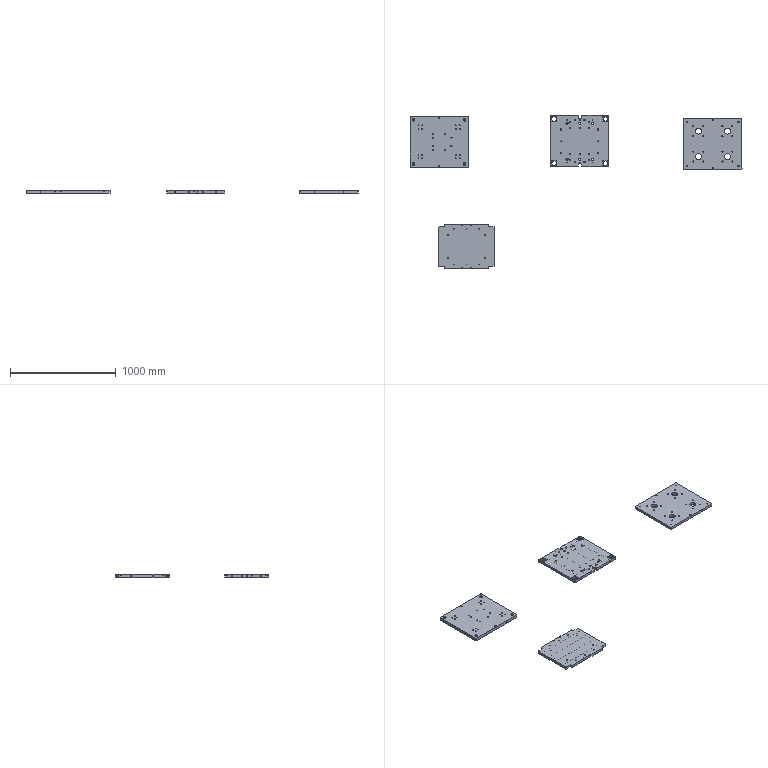CAM job | Mastercam | 3-axis milling, drilling | part box 3140 x 1452 x 30 mm
Tools:
tool_number,name,type,diameter_mm,corner_radius_mm,flutes,flute_length_mm,overall_length_mm,shoulder_length_mm,holder_diameter_mm,length_offset,diameter_offset,default_rpm,default_feed_mm_min,default_plunge_mm_min,coolant
1,11 Drill,drill,11,0,2,25,50,40,50,1,1,545,65.4,600,COOL_OFF
1,11 Drill,drill,11,0,2,25,50,40,50,1,1,545,65.4,600,COOL_OFF
1,11 Drill,drill,11,0,2,25,50,40,50,1,1,545,65.4,600,COOL_OFF
2,5.5 Drill,drill,5.5,0,2,25,50,40,50,2,2,1091,130.92,600,COOL_OFF
2,5.5 Drill,drill,5.5,0,2,25,50,40,50,2,2,1091,130.92,600,COOL_OFF
2,5.5 Drill,drill,5.5,0,2,25,50,40,50,2,2,1091,130.92,600,COOL_OFF
3,10.5 Drill,drill,10.5,0,2,25,50,40,50,3,3,571,68.52,600,COOL_OFF
3,10.5 Drill,drill,10.5,0,2,25,50,40,50,3,3,571,68.52,600,COOL_OFF
3,10.5 Drill,drill,10.5,0,2,25,50,40,50,3,3,571,68.52,600,COOL_OFF
5,5 Flat End Mill,end mill,5,0,4,25,75,25,50,5,5,2000,240,600,COOL_OFF
6,6 Flat End Mill,end mill,6,0,4,25,75,25,50,6,6,1667,200.04,600,COOL_OFF
6,6 Flat End Mill,end mill,6,0,4,25,75,25,50,6,6,1667,200.04,600,COOL_OFF
6,6 Flat End Mill,end mill,6,0,4,25,75,25,50,6,6,1667,200.04,600,COOL_OFF
7,4 Chamfer Mill,chamfer mill,4,0,4,25,75,30,50,7,7,6250,750,600,COOL_OFF
7,4 Chamfer Mill,chamfer mill,4,0,4,25,75,30,50,7,7,6250,750,600,COOL_OFF
7,4 Chamfer Mill,chamfer mill,4,0,4,25,75,30,50,7,7,6250,750,600,COOL_OFF
7,4 Chamfer Mill,chamfer mill,4,0,4,25,75,30,50,7,7,6250,750,600,COOL_OFF
8,8 Flat End Mill,end mill,8,0,4,25,75,25,50,8,8,1250,150,600,COOL_OFF
8,8 Flat End Mill,end mill,8,0,4,25,75,25,50,8,8,1250,150,600,COOL_OFF
8,8 Flat End Mill,end mill,8,0,4,25,75,25,50,8,8,1250,150,600,COOL_OFF
10,10 Flat End Mill,end mill,10,0,4,25,75,25,50,10,10,1005,120.6,600,COOL_OFF
12,12 Flat End Mill,end mill,12,0,4,25,75,25,50,12,12,833,99.96,600,COOL_OFF
12,12 Flat End Mill,end mill,12,0,4,25,75,25,50,12,12,833,99.96,600,COOL_OFF
12,12 Flat End Mill,end mill,12,0,4,25,75,25,50,12,12,833,99.96,600,COOL_OFF
13,10 Drill,drill,10,0,2,25,50,40,50,13,13,600,72,600,COOL_OFF
15,5.2 Drill,drill,5.2,0,2,25,50,40,50,15,15,1154,138.48,600,COOL_OFF
15,5.2 Drill,drill,5.2,0,2,25,50,40,50,15,15,1154,138.48,600,COOL_OFF
15,5.2 Drill,drill,5.2,0,2,25,50,40,50,15,15,1154,138.48,600,COOL_OFF
16,16 Flat End Mill,end mill,16,0,4,25,75,25,50,16,16,625,75,600,COOL_OFF
16,16 Flat End Mill,end mill,16,0,4,25,75,25,50,16,16,625,75,600,COOL_OFF
16,16 Flat End Mill,end mill,16,0,4,25,75,25,50,16,16,625,75,600,COOL_OFF
16,16 Flat End Mill,end mill,16,0,4,25,75,25,50,16,16,625,75,600,COOL_OFF
18,8.5 Drill,drill,8.5,0,2,25,50,40,50,18,18,706,84.72,600,COOL_OFF
19,9 Drill,drill,9,0,2,25,50,40,50,19,19,667,80.04,600,COOL_OFF
19,9 Drill,drill,9,0,2,25,50,40,50,19,19,667,80.04,600,COOL_OFF
24,100 Flat End Mill,end mill,100,0,4,25,75,25,50,24,24,100,12,600,COOL_OFF
Operations:
seq,operation,operation_type,tool_number,tool_name,tool_diameter_mm,spindle_rpm,feed_mm_min,plunge_mm_min,retract_mm_min,cycle_time_s,wcs,posted,nc_file
1,Manual Entry (吸),ManualEntry,,,,0,0,0,0,0,Plane,yes,1.nc
2,Contour (Ramp) - [WCS: Plane] - [Tplane: Plane],Contour,16,16 Flat End Mill,16,6000,4000,600,1200,935.276,Plane,yes,1.nc
3,Contour (2D) - [WCS: Plane] - [Tplane: Plane],Contour,12,12 Flat End Mill,12,6000,1000,600,1200,132.839,Plane,yes,1.nc
4,Contour (2D chamfer) - [WCS: Plane] - [Tplane: Plane],Contour,7,4 Chamfer Mill,4,6000,1000,600,1200,59.786,Plane,yes,1.nc
5,Manual Entry (clamp X),ManualEntry,,,,0,0,0,0,0,Plane,yes,1.nc
6,Manual Entry (M00),ManualEntry,,,,0,0,0,0,0,Plane,yes,1.nc
7,Contour (Ramp) - [WCS: Plane] - [Tplane: Plane],Contour,16,16 Flat End Mill,16,6000,4000,600,1200,785.449,Plane,yes,1.nc
8,Contour (2D) - [WCS: Plane] - [Tplane: Plane],Contour,12,12 Flat End Mill,12,6000,1000,600,1200,153.105,Plane,yes,1.nc
9,Contour (2D chamfer) - [WCS: Plane] - [Tplane: Plane],Contour,7,4 Chamfer Mill,4,6000,1000,600,1200,68.522,Plane,yes,1.nc
10,Drill/Counterbore - [WCS: Plane] - [Tplane: Plane],Drill,7,4 Chamfer Mill,4,6000,200,600,1200,29.657,Plane,yes,1.nc
11,Peck Drill - [WCS: Plane] - [Tplane: Plane],Drill,1,11 Drill,11,800,60,600,1200,202.333,Plane,yes,1.nc
12,Peck Drill - [WCS: Plane] - [Tplane: Plane],Drill,2,5.5 Drill,5.5,1200,100,600,1200,342.436,Plane,yes,1.nc
13,Peck Drill - [WCS: Plane] - [Tplane: Plane],Drill,3,10.5 Drill,10.5,800,80,600,1200,208.178,Plane,yes,1.nc
14,Contour (Ramp) - [WCS: Plane] - [Tplane: Plane],Contour,12,12 Flat End Mill,12,7000,3000,600,1200,66.499,Plane,yes,1.nc
15,Contour (2D) - [WCS: Plane] - [Tplane: Plane],Contour,12,12 Flat End Mill,12,7000,1000,600,1200,30.722,Plane,yes,1.nc
16,Contour (Ramp) - [WCS: Plane] - [Tplane: Plane],Contour,5,5 Flat End Mill,5,6000,2000,600,1200,222.229,Plane,yes,1.nc
17,Contour (Ramp) - [WCS: Plane] - [Tplane: Plane],Contour,5,5 Flat End Mill,5,6000,500,600,1200,108.808,Plane,yes,1.nc
18,Contour (2D chamfer) - [WCS: Plane] - [Tplane: Plane],Contour,7,4 Chamfer Mill,4,6000,1000,600,1200,94.527,Plane,yes,1.nc
19,Contour (2D chamfer) - [WCS: Plane] - [Tplane: Plane],Contour,7,4 Chamfer Mill,4,6000,1000,600,1200,25.86,Plane,yes,1.nc
20,Contour (Ramp) - [WCS: Plane-1] - [Tplane: Plane-1],Contour,8,8 Flat End Mill,8,7000,2000,600,1200,110.071,Plane-1,yes,1.nc
21,Contour (2D) - [WCS: Plane-1] - [Tplane: Plane-1],Contour,8,8 Flat End Mill,8,7000,1000,600,1200,21.213,Plane-1,yes,1.nc
22,Contour (2D chamfer) - [WCS: Plane-1] - [Tplane: Plane-1],Contour,7,4 Chamfer Mill,4,6000,1000,600,1200,36.511,Plane-1,yes,1.nc
23,Drill/Counterbore - [WCS: Plane-2] - [Tplane: Plane-2],Drill,7,4 Chamfer Mill,4,6000,200,600,1200,1.977,Plane-2,yes,1.nc
24,Peck Drill - [WCS: Plane-2] - [Tplane: Plane-2],Drill,15,5.2 Drill,5.2,1200,100,600,1200,32.506,Plane-2,yes,1.nc
25,Contour (2D chamfer) - [WCS: Plane-2] - [Tplane: Plane-2],Contour,7,4 Chamfer Mill,4,6000,1000,600,1200,2.903,Plane-2,yes,1.nc
26,Manual Entry (G91G28X0.Y0.),ManualEntry,,,,0,0,0,0,0,Plane-3,yes,1.nc
27,Drill/Counterbore - [WCS: Plane-3] - [Tplane: Plane-3],Drill,7,4 Chamfer Mill,4,6250,750,600,1200,1.383,Plane-3,yes,1.nc
28,Manual Entry (G91G28X0.Y0.),ManualEntry,,,,0,0,0,0,0,Plane-3,yes,1.nc
29,Peck Drill - [WCS: Plane-3] - [Tplane: Plane-3],Drill,15,5.2 Drill,5.2,1200,100,600,1200,86.688,Plane-3,yes,1.nc
30,Manual Entry (G91G28X0.Y0.),ManualEntry,,,,0,0,0,0,0,Plane-3,yes,1.nc
31,Contour (2D chamfer) - [WCS: Plane-3] - [Tplane: Plane-3],Contour,7,4 Chamfer Mill,4,6000,1000,600,1200,6.405,Plane-3,yes,1.nc
32,Manual Entry (吸),ManualEntry,,,,0,0,0,0,0,Plane-4,yes,3.nc
33,Contour (Ramp) - [WCS: Plane-4] - [Tplane: Plane-4],Contour,16,16 Flat End Mill,16,6000,4000,600,1200,772.88,Plane-4,yes,3.nc
34,Contour (2D) - [WCS: Plane-4] - [Tplane: Plane-4],Contour,12,12 Flat End Mill,12,6000,1000,600,1200,134.725,Plane-4,yes,3.nc
35,Contour (2D chamfer) - [WCS: Plane-4] - [Tplane: Plane-4],Contour,7,4 Chamfer Mill,4,6000,1000,600,1200,59.508,Plane-4,yes,3.nc
36,Manual Entry (clamp x),ManualEntry,,,,0,0,0,0,0,Plane-4,yes,3.nc
37,Manual Entry (M00),ManualEntry,,,,0,0,0,0,0,Plane-4,yes,3.nc
38,Contour (Ramp) - [WCS: Plane-4] - [Tplane: Plane-4],Contour,16,16 Flat End Mill,16,6000,4000,600,1200,81.512,Plane-4,yes,3.nc
39,Contour (Ramp) - [WCS: Plane-4] - [Tplane: Plane-4],Contour,16,16 Flat End Mill,16,6000,4000,600,1200,694.57,Plane-4,yes,3.nc
40,Contour (2D) - [WCS: Plane-4] - [Tplane: Plane-4],Contour,12,12 Flat End Mill,12,7000,1000,600,1200,163.475,Plane-4,yes,3.nc
41,Contour (2D chamfer) - [WCS: Plane-4] - [Tplane: Plane-4],Contour,7,4 Chamfer Mill,4,6000,1000,600,1200,74.224,Plane-4,yes,3.nc
42,2D High Speed (2D Dynamic Mill) - [WCS: Plane-4] - [Tplane: Plane-4],HighSpeed2D,16,16 Flat End Mill,16,6000,3000,600,1200,275.86,Plane-4,yes,3.nc
43,Contour (2D) - [WCS: Plane-4] - [Tplane: Plane-4],Contour,12,12 Flat End Mill,12,6000,1000,600,1200,65.773,Plane-4,yes,3.nc
44,Contour (Ramp) - [WCS: Plane-4] - [Tplane: Plane-4],Contour,12,12 Flat End Mill,12,6000,2000,600,1200,178.154,Plane-4,yes,3.nc
45,Contour (2D) - [WCS: Plane-4] - [Tplane: Plane-4],Contour,12,12 Flat End Mill,12,6000,1000,600,1200,43.243,Plane-4,yes,3.nc
46,Contour (Ramp) - [WCS: Plane-4] - [Tplane: Plane-4],Contour,6,6 Flat End Mill,6,6000,1500,600,1200,436.153,Plane-4,yes,3.nc
47,Contour (Ramp) - [WCS: Plane-4] - [Tplane: Plane-4],Contour,6,6 Flat End Mill,6,6000,500,600,1200,234.401,Plane-4,yes,3.nc
48,Drill/Counterbore - [WCS: Plane-4] - [Tplane: Plane-4],Drill,7,4 Chamfer Mill,4,6000,200,600,1200,33.611,Plane-4,yes,3.nc
49,Peck Drill - [WCS: Plane-4] - [Tplane: Plane-4],Drill,15,5.2 Drill,5.2,1200,100,600,1200,421.724,Plane-4,yes,3.nc
50,Peck Drill - [WCS: Plane-4] - [Tplane: Plane-4],Drill,3,10.5 Drill,10.5,800,80,600,1200,214.418,Plane-4,yes,3.nc
51,Contour (2D chamfer) - [WCS: Plane-4] - [Tplane: Plane-4],Contour,7,4 Chamfer Mill,4,6000,1000,600,1200,148.748,Plane-4,yes,3.nc
52,Drill/Counterbore - [WCS: Plane-5] - [Tplane: Plane-5],Drill,7,4 Chamfer Mill,4,6000,200,600,1200,3.954,Plane-5,yes,3.nc
53,Peck Drill - [WCS: Plane-5] - [Tplane: Plane-5],Drill,19,9 Drill,9,800,80,600,1200,180.821,Plane-5,yes,3.nc
54,Contour (2D chamfer) - [WCS: Plane-5] - [Tplane: Plane-5],Contour,7,4 Chamfer Mill,4,6000,1000,600,1200,9.139,Plane-5,yes,3.nc
55,Manual Entry (吸),ManualEntry,,,,0,0,0,0,0,Plane-6,yes,4.nc
56,Facing - [WCS: Plane-6] - [Tplane: Plane-6],Facing,24,100 Flat End Mill,100,4000,1000,600,1200,296.412,Plane-6,no,
57,Contour (Ramp) - [WCS: Plane-6] - [Tplane: Plane-6],Contour,16,16 Flat End Mill,16,6000,4000,600,1200,779.068,Plane-6,yes,4.nc
58,Contour (2D) - [WCS: Plane-6] - [Tplane: Plane-6],Contour,12,12 Flat End Mill,12,7000,1000,600,1200,131.767,Plane-6,yes,4.nc
59,Contour (2D chamfer) - [WCS: Plane-6] - [Tplane: Plane-6],Contour,7,4 Chamfer Mill,4,7000,1000,600,1200,59.786,Plane-6,yes,4.nc
60,Manual Entry (clamp X),ManualEntry,,,,0,0,0,0,0,Plane-6,yes,4.nc
61,Manual Entry (M00),ManualEntry,,,,0,0,0,0,0,Plane-6,yes,4.nc
62,Contour (Ramp) - [WCS: Plane-6] - [Tplane: Plane-6],Contour,16,16 Flat End Mill,16,6000,4000,600,1200,642.95,Plane-6,yes,4.nc
63,Contour (2D) - [WCS: Plane-6] - [Tplane: Plane-6],Contour,12,12 Flat End Mill,12,6000,1000,600,1200,152.033,Plane-6,yes,4.nc
64,Contour (2D chamfer) - [WCS: Plane-6] - [Tplane: Plane-6],Contour,7,4 Chamfer Mill,4,6000,1000,600,1200,68.522,Plane-6,yes,4.nc
65,2D High Speed (2D Dynamic Mill) - [WCS: Plane-6] - [Tplane: Plane-6],HighSpeed2D,16,16 Flat End Mill,16,6000,4000,600,1200,282.553,Plane-6,yes,4.nc
66,Drill/Counterbore - [WCS: Plane-6] - [Tplane: Plane-6],Drill,7,4 Chamfer Mill,4,6000,200,600,1200,21.748,Plane-6,yes,4.nc
67,Peck Drill - [WCS: Plane-6] - [Tplane: Plane-6],Drill,1,11 Drill,11,800,80,600,1200,128.651,Plane-6,yes,4.nc
68,Peck Drill - [WCS: Plane-6] - [Tplane: Plane-6],Drill,3,10.5 Drill,10.5,800,80,600,1200,343.069,Plane-6,yes,4.nc
69,Contour (2D) - [WCS: Plane-6] - [Tplane: Plane-6],Contour,12,12 Flat End Mill,12,6000,1000,600,1200,82.376,Plane-6,yes,4.nc
70,Contour (Ramp) - [WCS: Plane-6] - [Tplane: Plane-6],Contour,12,12 Flat End Mill,12,6000,3000,600,1200,67.227,Plane-6,yes,4.nc
71,Contour (2D) - [WCS: Plane-6] - [Tplane: Plane-6],Contour,12,12 Flat End Mill,12,6000,1000,600,1200,30.722,Plane-6,yes,4.nc
72,Contour (Ramp) - [WCS: Plane-6] - [Tplane: Plane-6],Contour,6,6 Flat End Mill,6,6000,2000,600,1200,58.432,Plane-6,yes,4.nc
73,Contour (Ramp) - [WCS: Plane-6] - [Tplane: Plane-6],Contour,6,6 Flat End Mill,6,6000,500,600,1200,29.617,Plane-6,yes,4.nc
74,Contour (2D chamfer) - [WCS: Plane-6] - [Tplane: Plane-6],Contour,7,4 Chamfer Mill,4,6000,1000,600,1200,123.493,Plane-6,yes,4.nc
75,Drill/Counterbore - [WCS: Plane-7] - [Tplane: Plane-7],Drill,7,4 Chamfer Mill,4,6000,200,600,1200,1.977,Plane-7,yes,4.nc
76,Peck Drill - [WCS: Plane-7] - [Tplane: Plane-7],Drill,15,5.2 Drill,5.2,1200,100,600,1200,32.506,Plane-7,yes,4.nc
77,Contour (2D chamfer) - [WCS: Plane-7] - [Tplane: Plane-7],Contour,7,4 Chamfer Mill,4,6000,1000,600,1200,3.175,Plane-7,yes,4.nc
78,Drill/Counterbore - [WCS: Plane-8] - [Tplane: Plane-8],Drill,7,4 Chamfer Mill,4,6000,200,600,1200,2.966,Plane-8,yes,4.nc
79,Peck Drill - [WCS: Plane-8] - [Tplane: Plane-8],Drill,15,5.2 Drill,5.2,1200,100,600,1200,48.758,Plane-8,yes,4.nc
80,Contour (2D chamfer) - [WCS: Plane-8] - [Tplane: Plane-8],Contour,7,4 Chamfer Mill,4,6000,1000,600,1200,4.763,Plane-8,yes,4.nc
81,Manual Entry (吸),ManualEntry,,,,0,0,0,0,0,Plane-9,yes,2.nc
82,Contour (Ramp) - [WCS: Plane-9] - [Tplane: Plane-9],Contour,16,16 Flat End Mill,16,6000,4000,600,1200,666.38,Plane-9,yes,2.nc
83,Contour (2D) - [WCS: Plane-9] - [Tplane: Plane-9],Contour,10,10 Flat End Mill,10,6000,1000,600,1200,114.508,Plane-9,yes,2.nc
84,Contour (2D chamfer) - [WCS: Plane-9] - [Tplane: Plane-9],Contour,7,4 Chamfer Mill,4,6000,1000,600,1200,51.708,Plane-9,yes,2.nc
85,Manual Entry (clamp X),ManualEntry,,,,0,0,0,0,0,Plane-9,yes,2.nc
86,Manual Entry (M00),ManualEntry,,,,0,0,0,0,0,Plane-9,yes,2.nc
87,Contour (Ramp) - [WCS: Plane-9] - [Tplane: Plane-9],Contour,16,16 Flat End Mill,16,6000,4000,600,1200,507.732,Plane-9,yes,2.nc
88,Contour (Ramp) - [WCS: Plane-9] - [Tplane: Plane-9],Contour,16,16 Flat End Mill,16,6000,4000,600,1200,657.767,Plane-9,yes,2.nc
89,Contour (Remachining) - [WCS: Plane-9] - [Tplane: Plane-9],Contour,10,10 Flat End Mill,10,6000,4000,600,1200,40.468,Plane-9,yes,2.nc
90,Contour (2D) - [WCS: Plane-9] - [Tplane: Plane-9],Contour,10,10 Flat End Mill,10,6000,1000,600,1200,154.716,Plane-9,yes,2.nc
91,Drill/Counterbore - [WCS: Plane-9] - [Tplane: Plane-9],Drill,7,4 Chamfer Mill,4,6000,200,600,1200,13.84,Plane-9,yes,2.nc
92,Peck Drill - [WCS: Plane-9] - [Tplane: Plane-9],Drill,18,8.5 Drill,8.5,800,100,600,1200,246.006,Plane-9,yes,2.nc
93,Contour (2D chamfer) - [WCS: Plane-9] - [Tplane: Plane-9],Contour,7,4 Chamfer Mill,4,6000,1000,600,1200,100.637,Plane-9,yes,2.nc
94,Drill/Counterbore - [WCS: Plane-10] - [Tplane: Plane-10],Drill,7,4 Chamfer Mill,4,6000,200,600,1200,4.943,Plane-10,yes,2.nc
95,Peck Drill - [WCS: Plane-10] - [Tplane: Plane-10],Drill,13,10 Drill,10,800,80,600,1200,180.821,Plane-10,yes,2.nc
96,Peck Drill - [WCS: Plane-10] - [Tplane: Plane-10],Drill,13,10 Drill,10,800,80,600,1200,21.593,Plane-10,yes,2.nc
97,Contour (Ramp) - [WCS: Plane-10] - [Tplane: Plane-10],Contour,6,6 Flat End Mill,6,6000,1000,600,1200,43.126,Plane-10,yes,2.nc
98,Contour (Ramp) - [WCS: Plane-10] - [Tplane: Plane-10],Contour,6,6 Flat End Mill,6,6000,500,600,1200,11.53,Plane-10,yes,2.nc
99,Contour (2D chamfer) - [WCS: Plane-10] - [Tplane: Plane-10],Contour,7,4 Chamfer Mill,4,6000,1000,600,1200,12.461,Plane-10,yes,2.nc